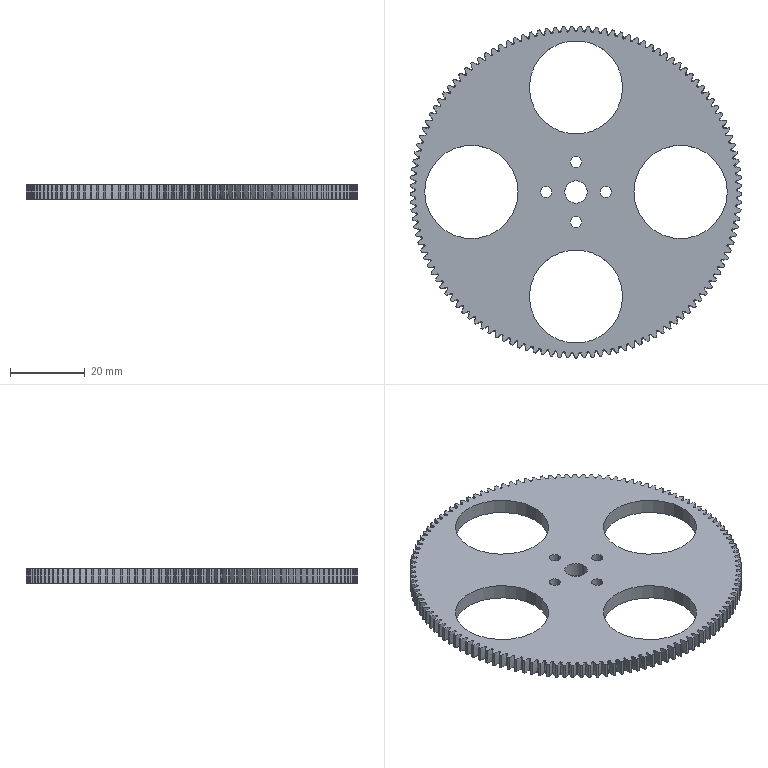Part | SolidWorks | features ICE 8, CirPattern 1, Extrusion 1, RefAxis 1 | 1 solid | 645 faces | box 88.898 x 88.892 x 4 mm | volume 15932 mm3 | cylinder 268 | spline 250 | plane 127 | commonest cylinder face diameters 85.749 x125 88.9 x125 3 x8 25 x8 6 x2